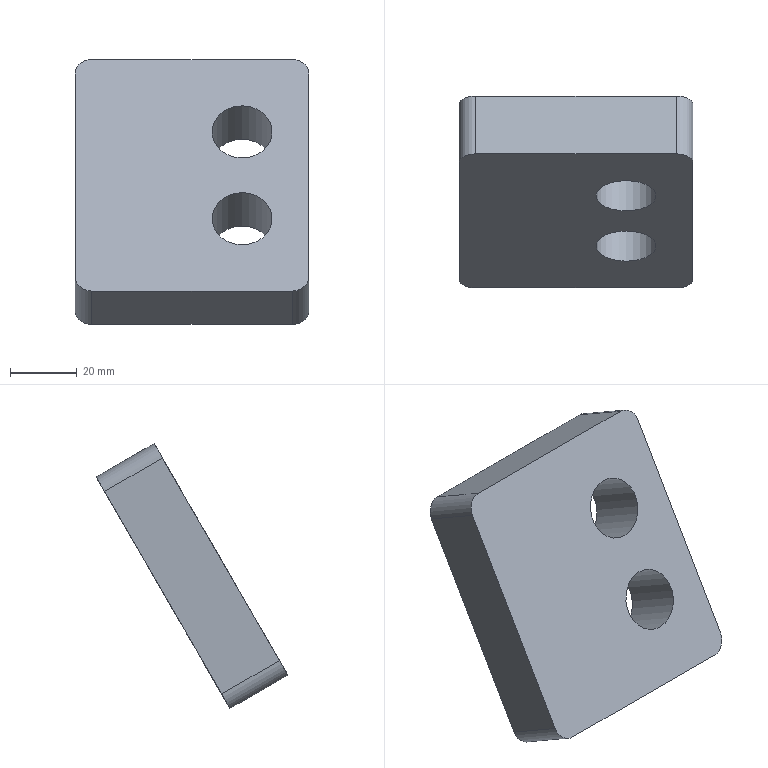Part | NX | features MAIN_BODY 2 | 1 solid | 12 faces | box 70 x 57.321 x 79.282 mm | volume 101392 mm3 | plane 6 | cylinder 6 | commonest cylinder face diameters 10 x4 18 x2
STEP:
#1=CARTESIAN_POINT('',(568.,453.094,-169.218));
#2=VERTEX_POINT('',#1);
#3=CARTESIAN_POINT('',(628.,453.094,-169.218));
#4=VERTEX_POINT('',#3);
#5=CARTESIAN_POINT('',(563.,453.094,-169.218));
#6=DIRECTION('',(1.,0.,0.));
#7=VECTOR('',#6,1000.);
#8=LINE('',#5,#7);
#9=EDGE_CURVE('',#2,#4,#8,.T.);
#10=ORIENTED_EDGE('',*,*,#9,.T.);
#11=CARTESIAN_POINT('',(628.,470.415,-179.218));
#12=VERTEX_POINT('',#11);
#13=CARTESIAN_POINT('',(628.,470.415,-179.218));
#14=DIRECTION('',(0.,-0.866,0.5));
#15=VECTOR('',#14,1000.);
#16=LINE('',#13,#15);
#17=EDGE_CURVE('',#12,#4,#16,.T.);
#18=ORIENTED_EDGE('',*,*,#17,.F.);
#19=CARTESIAN_POINT('',(568.,470.415,-179.218));
#20=VERTEX_POINT('',#19);
#21=CARTESIAN_POINT('',(563.,470.415,-179.218));
#22=DIRECTION('',(1.,0.,0.));
#23=VECTOR('',#22,1000.);
#24=LINE('',#21,#23);
#25=EDGE_CURVE('',#20,#12,#24,.T.);
#26=ORIENTED_EDGE('',*,*,#25,.F.);
#27=CARTESIAN_POINT('',(568.,470.415,-179.218));
#28=DIRECTION('',(0.,-0.866,0.5));
#29=VECTOR('',#28,1000.);
#30=LINE('',#27,#29);
#31=EDGE_CURVE('',#2,#20,#30,.F.);
#32=ORIENTED_EDGE('',*,*,#31,.F.);
#33=EDGE_LOOP('',(#10,#18,#26,#32));
#34=FACE_BOUND('',#33,.T.);
#35=CARTESIAN_POINT('',(563.,470.415,-179.218));
#36=DIRECTION('',(0.,0.5,0.866));
#37=DIRECTION('',(-1.,0.,0.));
#38=AXIS2_PLACEMENT_3D('',#35,#36,#37);
#39=PLANE('',#38);
#40=ADVANCED_FACE('',(#34),#39,.T.);
#41=CARTESIAN_POINT('',(633.,467.915,-183.548));
#42=VERTEX_POINT('',#41);
#43=CARTESIAN_POINT('',(633.,432.915,-244.17));
#44=VERTEX_POINT('',#43);
#45=CARTESIAN_POINT('',(633.,500.415,-127.256));
#46=DIRECTION('',(0.,-0.5,-0.866));
#47=VECTOR('',#46,1000.);
#48=LINE('',#45,#47);
#49=EDGE_CURVE('',#42,#44,#48,.T.);
#50=ORIENTED_EDGE('',*,*,#49,.F.);
#51=CARTESIAN_POINT('',(633.,450.594,-173.548));
#52=VERTEX_POINT('',#51);
#53=CARTESIAN_POINT('',(633.,467.915,-183.548));
#54=DIRECTION('',(0.,-0.866,0.5));
#55=VECTOR('',#54,1000.);
#56=LINE('',#53,#55);
#57=EDGE_CURVE('',#52,#42,#56,.F.);
#58=ORIENTED_EDGE('',*,*,#57,.F.);
#59=CARTESIAN_POINT('',(633.,415.594,-234.17));
#60=VERTEX_POINT('',#59);
#61=CARTESIAN_POINT('',(633.,483.094,-117.256));
#62=DIRECTION('',(0.,-0.5,-0.866));
#63=VECTOR('',#62,1000.);
#64=LINE('',#61,#63);
#65=EDGE_CURVE('',#52,#60,#64,.T.);
#66=ORIENTED_EDGE('',*,*,#65,.T.);
#67=CARTESIAN_POINT('',(633.,432.915,-244.17));
#68=DIRECTION('',(0.,-0.866,0.5));
#69=VECTOR('',#68,1000.);
#70=LINE('',#67,#69);
#71=EDGE_CURVE('',#44,#60,#70,.T.);
#72=ORIENTED_EDGE('',*,*,#71,.F.);
#73=EDGE_LOOP('',(#50,#58,#66,#72));
#74=FACE_BOUND('',#73,.T.);
#75=CARTESIAN_POINT('',(633.,500.415,-127.256));
#76=DIRECTION('',(1.,0.,0.));
#77=DIRECTION('',(0.,0.5,0.866));
#78=AXIS2_PLACEMENT_3D('',#75,#76,#77);
#79=PLANE('',#78);
#80=ADVANCED_FACE('',(#74),#79,.T.);
#81=CARTESIAN_POINT('',(628.,430.415,-248.5));
#82=VERTEX_POINT('',#81);
#83=CARTESIAN_POINT('',(568.,430.415,-248.5));
#84=VERTEX_POINT('',#83);
#85=CARTESIAN_POINT('',(633.,430.415,-248.5));
#86=DIRECTION('',(-1.,0.,0.));
#87=VECTOR('',#86,1000.);
#88=LINE('',#85,#87);
#89=EDGE_CURVE('',#82,#84,#88,.T.);
#90=ORIENTED_EDGE('',*,*,#89,.F.);
#91=CARTESIAN_POINT('',(628.,413.094,-238.5));
#92=VERTEX_POINT('',#91);
#93=CARTESIAN_POINT('',(628.,430.415,-248.5));
#94=DIRECTION('',(0.,-0.866,0.5));
#95=VECTOR('',#94,1000.);
#96=LINE('',#93,#95);
#97=EDGE_CURVE('',#92,#82,#96,.F.);
#98=ORIENTED_EDGE('',*,*,#97,.F.);
#99=CARTESIAN_POINT('',(568.,413.094,-238.5));
#100=VERTEX_POINT('',#99);
#101=CARTESIAN_POINT('',(633.,413.094,-238.5));
#102=DIRECTION('',(-1.,0.,0.));
#103=VECTOR('',#102,1000.);
#104=LINE('',#101,#103);
#105=EDGE_CURVE('',#92,#100,#104,.T.);
#106=ORIENTED_EDGE('',*,*,#105,.T.);
#107=CARTESIAN_POINT('',(568.,430.415,-248.5));
#108=DIRECTION('',(0.,-0.866,0.5));
#109=VECTOR('',#108,1000.);
#110=LINE('',#107,#109);
#111=EDGE_CURVE('',#84,#100,#110,.T.);
#112=ORIENTED_EDGE('',*,*,#111,.F.);
#113=EDGE_LOOP('',(#90,#98,#106,#112));
#114=FACE_BOUND('',#113,.T.);
#115=CARTESIAN_POINT('',(633.,430.415,-248.5));
#116=DIRECTION('',(0.,-0.5,-0.866));
#117=DIRECTION('',(0.,0.866,-0.5));
#118=AXIS2_PLACEMENT_3D('',#115,#116,#117);
#119=PLANE('',#118);
#120=ADVANCED_FACE('',(#114),#119,.T.);
#121=CARTESIAN_POINT('',(563.,415.594,-234.17));
#122=VERTEX_POINT('',#121);
#123=CARTESIAN_POINT('',(563.,450.594,-173.548));
#124=VERTEX_POINT('',#123);
#125=CARTESIAN_POINT('',(563.,403.094,-255.821));
#126=DIRECTION('',(0.,0.5,0.866));
#127=VECTOR('',#126,1000.);
#128=LINE('',#125,#127);
#129=EDGE_CURVE('',#122,#124,#128,.T.);
#130=ORIENTED_EDGE('',*,*,#129,.T.);
#131=CARTESIAN_POINT('',(563.,467.915,-183.548));
#132=VERTEX_POINT('',#131);
#133=CARTESIAN_POINT('',(563.,467.915,-183.548));
#134=DIRECTION('',(0.,-0.866,0.5));
#135=VECTOR('',#134,1000.);
#136=LINE('',#133,#135);
#137=EDGE_CURVE('',#132,#124,#136,.T.);
#138=ORIENTED_EDGE('',*,*,#137,.F.);
#139=CARTESIAN_POINT('',(563.,432.915,-244.17));
#140=VERTEX_POINT('',#139);
#141=CARTESIAN_POINT('',(563.,420.415,-265.821));
#142=DIRECTION('',(0.,0.5,0.866));
#143=VECTOR('',#142,1000.);
#144=LINE('',#141,#143);
#145=EDGE_CURVE('',#140,#132,#144,.T.);
#146=ORIENTED_EDGE('',*,*,#145,.F.);
#147=CARTESIAN_POINT('',(563.,432.915,-244.17));
#148=DIRECTION('',(0.,-0.866,0.5));
#149=VECTOR('',#148,1000.);
#150=LINE('',#147,#149);
#151=EDGE_CURVE('',#122,#140,#150,.F.);
#152=ORIENTED_EDGE('',*,*,#151,.F.);
#153=EDGE_LOOP('',(#130,#138,#146,#152));
#154=FACE_BOUND('',#153,.T.);
#155=CARTESIAN_POINT('',(563.,420.415,-265.821));
#156=DIRECTION('',(-1.,0.,0.));
#157=DIRECTION('',(0.,0.866,-0.5));
#158=AXIS2_PLACEMENT_3D('',#155,#156,#157);
#159=PLANE('',#158);
#160=ADVANCED_FACE('',(#154),#159,.T.);
#161=CARTESIAN_POINT('',(613.,438.415,-234.644));
#162=VERTEX_POINT('',#161);
#163=CARTESIAN_POINT('',(613.,442.915,-226.849));
#164=DIRECTION('',(0.,0.866,-0.5));
#165=DIRECTION('',(0.,-0.5,-0.866));
#166=AXIS2_PLACEMENT_3D('',#163,#164,#165);
#167=CIRCLE('',#166,9.);
#168=EDGE_CURVE('',#162,#162,#167,.T.);
#169=ORIENTED_EDGE('',*,*,#168,.F.);
#170=EDGE_LOOP('',(#169));
#171=FACE_BOUND('',#170,.T.);
#172=CARTESIAN_POINT('',(613.,453.415,-208.663));
#173=VERTEX_POINT('',#172);
#174=CARTESIAN_POINT('',(613.,457.915,-200.869));
#175=DIRECTION('',(0.,0.866,-0.5));
#176=DIRECTION('',(0.,-0.5,-0.866));
#177=AXIS2_PLACEMENT_3D('',#174,#175,#176);
#178=CIRCLE('',#177,9.);
#179=EDGE_CURVE('',#173,#173,#178,.T.);
#180=ORIENTED_EDGE('',*,*,#179,.F.);
#181=EDGE_LOOP('',(#180));
#182=FACE_BOUND('',#181,.T.);
#183=ORIENTED_EDGE('',*,*,#145,.T.);
#184=CARTESIAN_POINT('',(568.,467.915,-183.548));
#185=DIRECTION('',(0.,0.866,-0.5));
#186=DIRECTION('',(0.,-0.5,-0.866));
#187=AXIS2_PLACEMENT_3D('',#184,#185,#186);
#188=CIRCLE('',#187,5.);
#189=EDGE_CURVE('',#20,#132,#188,.F.);
#190=ORIENTED_EDGE('',*,*,#189,.F.);
#191=ORIENTED_EDGE('',*,*,#25,.T.);
#192=CARTESIAN_POINT('',(628.,467.915,-183.548));
#193=DIRECTION('',(0.,0.866,-0.5));
#194=DIRECTION('',(0.,-0.5,-0.866));
#195=AXIS2_PLACEMENT_3D('',#192,#193,#194);
#196=CIRCLE('',#195,5.);
#197=EDGE_CURVE('',#42,#12,#196,.F.);
#198=ORIENTED_EDGE('',*,*,#197,.F.);
#199=ORIENTED_EDGE('',*,*,#49,.T.);
#200=CARTESIAN_POINT('',(628.,432.915,-244.17));
#201=DIRECTION('',(0.,0.866,-0.5));
#202=DIRECTION('',(0.,-0.5,-0.866));
#203=AXIS2_PLACEMENT_3D('',#200,#201,#202);
#204=CIRCLE('',#203,5.);
#205=EDGE_CURVE('',#82,#44,#204,.F.);
#206=ORIENTED_EDGE('',*,*,#205,.F.);
#207=ORIENTED_EDGE('',*,*,#89,.T.);
#208=CARTESIAN_POINT('',(568.,432.915,-244.17));
#209=DIRECTION('',(0.,0.866,-0.5));
#210=DIRECTION('',(0.,-0.5,-0.866));
#211=AXIS2_PLACEMENT_3D('',#208,#209,#210);
#212=CIRCLE('',#211,5.);
#213=EDGE_CURVE('',#140,#84,#212,.F.);
#214=ORIENTED_EDGE('',*,*,#213,.F.);
#215=EDGE_LOOP('',(#183,#190,#191,#198,#199,#206,#207,#214));
#216=FACE_BOUND('',#215,.T.);
#217=CARTESIAN_POINT('',(633.,500.415,-127.256));
#218=DIRECTION('',(0.,-0.866,0.5));
#219=DIRECTION('',(0.,-0.5,-0.866));
#220=AXIS2_PLACEMENT_3D('',#217,#218,#219);
#221=PLANE('',#220);
#222=ADVANCED_FACE('',(#171,#182,#216),#221,.F.);
#223=CARTESIAN_POINT('',(613.,421.094,-224.644));
#224=VERTEX_POINT('',#223);
#225=CARTESIAN_POINT('',(613.,425.594,-216.849));
#226=DIRECTION('',(0.,-0.866,0.5));
#227=DIRECTION('',(0.,-0.5,-0.866));
#228=AXIS2_PLACEMENT_3D('',#225,#226,#227);
#229=CIRCLE('',#228,9.);
#230=EDGE_CURVE('',#224,#224,#229,.F.);
#231=ORIENTED_EDGE('',*,*,#230,.T.);
#232=EDGE_LOOP('',(#231));
#233=FACE_BOUND('',#232,.T.);
#234=CARTESIAN_POINT('',(613.,436.094,-198.663));
#235=VERTEX_POINT('',#234);
#236=CARTESIAN_POINT('',(613.,440.594,-190.869));
#237=DIRECTION('',(0.,-0.866,0.5));
#238=DIRECTION('',(0.,-0.5,-0.866));
#239=AXIS2_PLACEMENT_3D('',#236,#237,#238);
#240=CIRCLE('',#239,9.);
#241=EDGE_CURVE('',#235,#235,#240,.F.);
#242=ORIENTED_EDGE('',*,*,#241,.T.);
#243=EDGE_LOOP('',(#242));
#244=FACE_BOUND('',#243,.T.);
#245=ORIENTED_EDGE('',*,*,#105,.F.);
#246=CARTESIAN_POINT('',(628.,415.594,-234.17));
#247=DIRECTION('',(0.,-0.866,0.5));
#248=DIRECTION('',(0.,-0.5,-0.866));
#249=AXIS2_PLACEMENT_3D('',#246,#247,#248);
#250=CIRCLE('',#249,5.);
#251=EDGE_CURVE('',#60,#92,#250,.F.);
#252=ORIENTED_EDGE('',*,*,#251,.F.);
#253=ORIENTED_EDGE('',*,*,#65,.F.);
#254=CARTESIAN_POINT('',(628.,450.594,-173.548));
#255=DIRECTION('',(0.,-0.866,0.5));
#256=DIRECTION('',(0.,-0.5,-0.866));
#257=AXIS2_PLACEMENT_3D('',#254,#255,#256);
#258=CIRCLE('',#257,5.);
#259=EDGE_CURVE('',#4,#52,#258,.F.);
#260=ORIENTED_EDGE('',*,*,#259,.F.);
#261=ORIENTED_EDGE('',*,*,#9,.F.);
#262=CARTESIAN_POINT('',(568.,450.594,-173.548));
#263=DIRECTION('',(0.,-0.866,0.5));
#264=DIRECTION('',(0.,-0.5,-0.866));
#265=AXIS2_PLACEMENT_3D('',#262,#263,#264);
#266=CIRCLE('',#265,5.);
#267=EDGE_CURVE('',#124,#2,#266,.F.);
#268=ORIENTED_EDGE('',*,*,#267,.F.);
#269=ORIENTED_EDGE('',*,*,#129,.F.);
#270=CARTESIAN_POINT('',(568.,415.594,-234.17));
#271=DIRECTION('',(0.,-0.866,0.5));
#272=DIRECTION('',(0.,-0.5,-0.866));
#273=AXIS2_PLACEMENT_3D('',#270,#271,#272);
#274=CIRCLE('',#273,5.);
#275=EDGE_CURVE('',#100,#122,#274,.F.);
#276=ORIENTED_EDGE('',*,*,#275,.F.);
#277=EDGE_LOOP('',(#245,#252,#253,#260,#261,#268,#269,#276));
#278=FACE_BOUND('',#277,.T.);
#279=CARTESIAN_POINT('',(633.,483.094,-117.256));
#280=DIRECTION('',(0.,-0.866,0.5));
#281=DIRECTION('',(0.,-0.5,-0.866));
#282=AXIS2_PLACEMENT_3D('',#279,#280,#281);
#283=PLANE('',#282);
#284=ADVANCED_FACE('',(#233,#244,#278),#283,.T.);
#285=ORIENTED_EDGE('',*,*,#241,.F.);
#286=EDGE_LOOP('',(#285));
#287=FACE_BOUND('',#286,.T.);
#288=ORIENTED_EDGE('',*,*,#179,.T.);
#289=EDGE_LOOP('',(#288));
#290=FACE_BOUND('',#289,.T.);
#291=CARTESIAN_POINT('',(613.,457.915,-200.869));
#292=DIRECTION('',(0.,-0.866,0.5));
#293=DIRECTION('',(0.,-0.5,-0.866));
#294=AXIS2_PLACEMENT_3D('',#291,#292,#293);
#295=CYLINDRICAL_SURFACE('',#294,9.);
#296=ADVANCED_FACE('',(#287,#290),#295,.F.);
#297=ORIENTED_EDGE('',*,*,#230,.F.);
#298=EDGE_LOOP('',(#297));
#299=FACE_BOUND('',#298,.T.);
#300=ORIENTED_EDGE('',*,*,#168,.T.);
#301=EDGE_LOOP('',(#300));
#302=FACE_BOUND('',#301,.T.);
#303=CARTESIAN_POINT('',(613.,442.915,-226.849));
#304=DIRECTION('',(0.,-0.866,0.5));
#305=DIRECTION('',(0.,-0.5,-0.866));
#306=AXIS2_PLACEMENT_3D('',#303,#304,#305);
#307=CYLINDRICAL_SURFACE('',#306,9.);
#308=ADVANCED_FACE('',(#299,#302),#307,.F.);
#309=ORIENTED_EDGE('',*,*,#213,.T.);
#310=ORIENTED_EDGE('',*,*,#111,.T.);
#311=ORIENTED_EDGE('',*,*,#275,.T.);
#312=ORIENTED_EDGE('',*,*,#151,.T.);
#313=EDGE_LOOP('',(#309,#310,#311,#312));
#314=FACE_BOUND('',#313,.T.);
#315=CARTESIAN_POINT('',(568.,432.915,-244.17));
#316=DIRECTION('',(0.,-0.866,0.5));
#317=DIRECTION('',(0.,-0.5,-0.866));
#318=AXIS2_PLACEMENT_3D('',#315,#316,#317);
#319=CYLINDRICAL_SURFACE('',#318,5.);
#320=ADVANCED_FACE('',(#314),#319,.T.);
#321=ORIENTED_EDGE('',*,*,#205,.T.);
#322=ORIENTED_EDGE('',*,*,#71,.T.);
#323=ORIENTED_EDGE('',*,*,#251,.T.);
#324=ORIENTED_EDGE('',*,*,#97,.T.);
#325=EDGE_LOOP('',(#321,#322,#323,#324));
#326=FACE_BOUND('',#325,.T.);
#327=CARTESIAN_POINT('',(628.,432.915,-244.17));
#328=DIRECTION('',(0.,-0.866,0.5));
#329=DIRECTION('',(0.,-0.5,-0.866));
#330=AXIS2_PLACEMENT_3D('',#327,#328,#329);
#331=CYLINDRICAL_SURFACE('',#330,5.);
#332=ADVANCED_FACE('',(#326),#331,.T.);
#333=ORIENTED_EDGE('',*,*,#189,.T.);
#334=ORIENTED_EDGE('',*,*,#137,.T.);
#335=ORIENTED_EDGE('',*,*,#267,.T.);
#336=ORIENTED_EDGE('',*,*,#31,.T.);
#337=EDGE_LOOP('',(#333,#334,#335,#336));
#338=FACE_BOUND('',#337,.T.);
#339=CARTESIAN_POINT('',(568.,467.915,-183.548));
#340=DIRECTION('',(0.,-0.866,0.5));
#341=DIRECTION('',(0.,-0.5,-0.866));
#342=AXIS2_PLACEMENT_3D('',#339,#340,#341);
#343=CYLINDRICAL_SURFACE('',#342,5.);
#344=ADVANCED_FACE('',(#338),#343,.T.);
#345=ORIENTED_EDGE('',*,*,#197,.T.);
#346=ORIENTED_EDGE('',*,*,#17,.T.);
#347=ORIENTED_EDGE('',*,*,#259,.T.);
#348=ORIENTED_EDGE('',*,*,#57,.T.);
#349=EDGE_LOOP('',(#345,#346,#347,#348));
#350=FACE_BOUND('',#349,.T.);
#351=CARTESIAN_POINT('',(628.,467.915,-183.548));
#352=DIRECTION('',(0.,-0.866,0.5));
#353=DIRECTION('',(0.,-0.5,-0.866));
#354=AXIS2_PLACEMENT_3D('',#351,#352,#353);
#355=CYLINDRICAL_SURFACE('',#354,5.);
#356=ADVANCED_FACE('',(#350),#355,.T.);
#357=CLOSED_SHELL('',(#40,#80,#120,#160,#222,#284,#296,#308,#320,#332,#344,#356));
#358=MANIFOLD_SOLID_BREP('',#357);
#359=(LENGTH_UNIT()NAMED_UNIT(*)SI_UNIT(.MILLI.,.METRE.));
#360=UNCERTAINTY_MEASURE_WITH_UNIT(LENGTH_MEASURE(0.00001),#359,'','');
#361=(NAMED_UNIT(*)PLANE_ANGLE_UNIT()SI_UNIT($,.RADIAN.));
#362=(NAMED_UNIT(*)SI_UNIT($,.STERADIAN.)SOLID_ANGLE_UNIT());
#363=(GEOMETRIC_REPRESENTATION_CONTEXT(3)GLOBAL_UNCERTAINTY_ASSIGNED_CONTEXT((#360))GLOBAL_UNIT_ASSIGNED_CONTEXT((#359,#361,#362))REPRESENTATION_CONTEXT('',''));
#364=ADVANCED_BREP_SHAPE_REPRESENTATION('',(#358),#363);